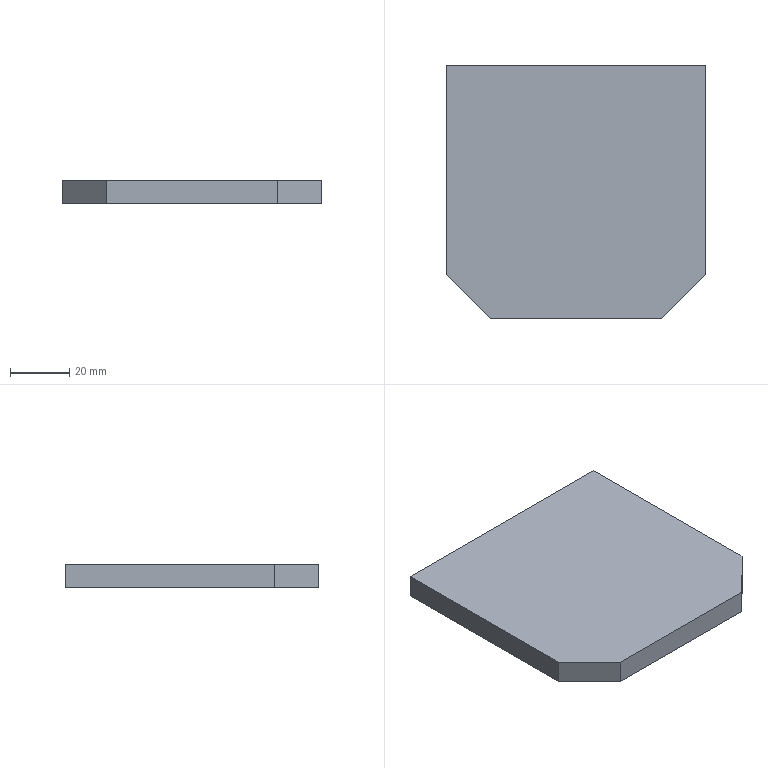Part | STEP file | 400 | 1 solid | 8 faces | box 88 x 86 x 8 mm | volume 58744 mm3 | plane 8
STEP:
#1=CARTESIAN_POINT('',(-29.,-94.,725.));
#2=VERTEX_POINT('',#1);
#3=CARTESIAN_POINT('',(-29.,-94.,717.));
#4=VERTEX_POINT('',#3);
#5=CARTESIAN_POINT('',(-29.,-94.,725.));
#6=DIRECTION('',(0.,0.,-1.));
#7=VECTOR('',#6,1000.);
#8=LINE('',#5,#7);
#9=EDGE_CURVE('',#2,#4,#8,.T.);
#10=ORIENTED_EDGE('',*,*,#9,.T.);
#11=CARTESIAN_POINT('',(29.,-94.,717.));
#12=VERTEX_POINT('',#11);
#13=CARTESIAN_POINT('',(-29.,-94.,717.));
#14=DIRECTION('',(1.,0.,0.));
#15=VECTOR('',#14,1000.);
#16=LINE('',#13,#15);
#17=EDGE_CURVE('',#4,#12,#16,.T.);
#18=ORIENTED_EDGE('',*,*,#17,.T.);
#19=CARTESIAN_POINT('',(29.,-94.,725.));
#20=VERTEX_POINT('',#19);
#21=CARTESIAN_POINT('',(29.,-94.,725.));
#22=DIRECTION('',(0.,0.,-1.));
#23=VECTOR('',#22,1000.);
#24=LINE('',#21,#23);
#25=EDGE_CURVE('',#20,#12,#24,.T.);
#26=ORIENTED_EDGE('',*,*,#25,.F.);
#27=CARTESIAN_POINT('',(-29.,-94.,725.));
#28=DIRECTION('',(1.,0.,0.));
#29=VECTOR('',#28,1000.);
#30=LINE('',#27,#29);
#31=EDGE_CURVE('',#2,#20,#30,.T.);
#32=ORIENTED_EDGE('',*,*,#31,.F.);
#33=EDGE_LOOP('',(#10,#18,#26,#32));
#34=FACE_OUTER_BOUND('',#33,.T.);
#35=CARTESIAN_POINT('',(-29.,-94.,717.));
#36=DIRECTION('',(0.,-1.,0.));
#37=DIRECTION('',(0.,0.,-1.));
#38=AXIS2_PLACEMENT_3D('',#35,#36,#37);
#39=PLANE('',#38);
#40=ADVANCED_FACE('',(#34),#39,.T.);
#41=CARTESIAN_POINT('',(-44.,-79.,725.));
#42=VERTEX_POINT('',#41);
#43=CARTESIAN_POINT('',(-44.,-79.,717.));
#44=VERTEX_POINT('',#43);
#45=CARTESIAN_POINT('',(-44.,-79.,725.));
#46=DIRECTION('',(0.,0.,-1.));
#47=VECTOR('',#46,1000.);
#48=LINE('',#45,#47);
#49=EDGE_CURVE('',#42,#44,#48,.T.);
#50=ORIENTED_EDGE('',*,*,#49,.T.);
#51=CARTESIAN_POINT('',(-29.,-94.,717.));
#52=DIRECTION('',(-0.7071,0.7071,0.));
#53=VECTOR('',#52,1000.);
#54=LINE('',#51,#53);
#55=EDGE_CURVE('',#4,#44,#54,.T.);
#56=ORIENTED_EDGE('',*,*,#55,.F.);
#57=ORIENTED_EDGE('',*,*,#9,.F.);
#58=CARTESIAN_POINT('',(-44.,-79.,725.));
#59=DIRECTION('',(0.7071,-0.7071,0.));
#60=VECTOR('',#59,1000.);
#61=LINE('',#58,#60);
#62=EDGE_CURVE('',#42,#2,#61,.T.);
#63=ORIENTED_EDGE('',*,*,#62,.F.);
#64=EDGE_LOOP('',(#50,#56,#57,#63));
#65=FACE_OUTER_BOUND('',#64,.T.);
#66=CARTESIAN_POINT('',(-44.,-79.,717.));
#67=DIRECTION('',(-0.7071,-0.7071,0.));
#68=DIRECTION('',(-0.7071,0.7071,0.));
#69=AXIS2_PLACEMENT_3D('',#66,#67,#68);
#70=PLANE('',#69);
#71=ADVANCED_FACE('',(#65),#70,.T.);
#72=CARTESIAN_POINT('',(44.,-79.,725.));
#73=VERTEX_POINT('',#72);
#74=CARTESIAN_POINT('',(44.,-79.,717.));
#75=VERTEX_POINT('',#74);
#76=CARTESIAN_POINT('',(44.,-79.,725.));
#77=DIRECTION('',(0.,0.,-1.));
#78=VECTOR('',#77,1000.);
#79=LINE('',#76,#78);
#80=EDGE_CURVE('',#73,#75,#79,.T.);
#81=ORIENTED_EDGE('',*,*,#80,.T.);
#82=CARTESIAN_POINT('',(44.,-8.,717.));
#83=VERTEX_POINT('',#82);
#84=CARTESIAN_POINT('',(44.,-8.,717.));
#85=DIRECTION('',(0.,-1.,0.));
#86=VECTOR('',#85,1000.);
#87=LINE('',#84,#86);
#88=EDGE_CURVE('',#83,#75,#87,.T.);
#89=ORIENTED_EDGE('',*,*,#88,.F.);
#90=CARTESIAN_POINT('',(44.,-8.,725.));
#91=VERTEX_POINT('',#90);
#92=CARTESIAN_POINT('',(44.,-8.,725.));
#93=DIRECTION('',(0.,0.,-1.));
#94=VECTOR('',#93,1000.);
#95=LINE('',#92,#94);
#96=EDGE_CURVE('',#91,#83,#95,.T.);
#97=ORIENTED_EDGE('',*,*,#96,.F.);
#98=CARTESIAN_POINT('',(44.,-79.,725.));
#99=DIRECTION('',(0.,1.,0.));
#100=VECTOR('',#99,1000.);
#101=LINE('',#98,#100);
#102=EDGE_CURVE('',#73,#91,#101,.T.);
#103=ORIENTED_EDGE('',*,*,#102,.F.);
#104=EDGE_LOOP('',(#81,#89,#97,#103));
#105=FACE_OUTER_BOUND('',#104,.T.);
#106=CARTESIAN_POINT('',(44.,-79.,717.));
#107=DIRECTION('',(1.,0.,0.));
#108=DIRECTION('',(0.,1.,0.));
#109=AXIS2_PLACEMENT_3D('',#106,#107,#108);
#110=PLANE('',#109);
#111=ADVANCED_FACE('',(#105),#110,.T.);
#112=ORIENTED_EDGE('',*,*,#96,.T.);
#113=CARTESIAN_POINT('',(-44.,-8.,717.));
#114=VERTEX_POINT('',#113);
#115=CARTESIAN_POINT('',(-44.,-8.,717.));
#116=DIRECTION('',(1.,0.,0.));
#117=VECTOR('',#116,1000.);
#118=LINE('',#115,#117);
#119=EDGE_CURVE('',#114,#83,#118,.T.);
#120=ORIENTED_EDGE('',*,*,#119,.F.);
#121=CARTESIAN_POINT('',(-44.,-8.,725.));
#122=VERTEX_POINT('',#121);
#123=CARTESIAN_POINT('',(-44.,-8.,725.));
#124=DIRECTION('',(0.,0.,-1.));
#125=VECTOR('',#124,1000.);
#126=LINE('',#123,#125);
#127=EDGE_CURVE('',#122,#114,#126,.T.);
#128=ORIENTED_EDGE('',*,*,#127,.F.);
#129=CARTESIAN_POINT('',(44.,-8.,725.));
#130=DIRECTION('',(-1.,0.,0.));
#131=VECTOR('',#130,1000.);
#132=LINE('',#129,#131);
#133=EDGE_CURVE('',#91,#122,#132,.T.);
#134=ORIENTED_EDGE('',*,*,#133,.F.);
#135=EDGE_LOOP('',(#112,#120,#128,#134));
#136=FACE_OUTER_BOUND('',#135,.T.);
#137=CARTESIAN_POINT('',(29.,-8.,717.));
#138=DIRECTION('',(0.,1.,0.));
#139=DIRECTION('',(1.,0.,0.));
#140=AXIS2_PLACEMENT_3D('',#137,#138,#139);
#141=PLANE('',#140);
#142=ADVANCED_FACE('',(#136),#141,.T.);
#143=ORIENTED_EDGE('',*,*,#88,.T.);
#144=CARTESIAN_POINT('',(44.,-79.,717.));
#145=DIRECTION('',(-0.7071,-0.7071,0.));
#146=VECTOR('',#145,1000.);
#147=LINE('',#144,#146);
#148=EDGE_CURVE('',#75,#12,#147,.T.);
#149=ORIENTED_EDGE('',*,*,#148,.T.);
#150=ORIENTED_EDGE('',*,*,#17,.F.);
#151=ORIENTED_EDGE('',*,*,#55,.T.);
#152=CARTESIAN_POINT('',(-44.,-8.,717.));
#153=DIRECTION('',(0.,-1.,0.));
#154=VECTOR('',#153,1000.);
#155=LINE('',#152,#154);
#156=EDGE_CURVE('',#114,#44,#155,.T.);
#157=ORIENTED_EDGE('',*,*,#156,.F.);
#158=ORIENTED_EDGE('',*,*,#119,.T.);
#159=EDGE_LOOP('',(#143,#149,#150,#151,#157,#158));
#160=FACE_OUTER_BOUND('',#159,.T.);
#161=CARTESIAN_POINT('',(0.,0.,717.));
#162=DIRECTION('',(0.,0.,-1.));
#163=DIRECTION('',(0.,-1.,0.));
#164=AXIS2_PLACEMENT_3D('',#161,#162,#163);
#165=PLANE('',#164);
#166=ADVANCED_FACE('',(#160),#165,.T.);
#167=ORIENTED_EDGE('',*,*,#49,.F.);
#168=CARTESIAN_POINT('',(-44.,-8.,725.));
#169=DIRECTION('',(0.,-1.,0.));
#170=VECTOR('',#169,1000.);
#171=LINE('',#168,#170);
#172=EDGE_CURVE('',#122,#42,#171,.T.);
#173=ORIENTED_EDGE('',*,*,#172,.F.);
#174=ORIENTED_EDGE('',*,*,#127,.T.);
#175=ORIENTED_EDGE('',*,*,#156,.T.);
#176=EDGE_LOOP('',(#167,#173,#174,#175));
#177=FACE_OUTER_BOUND('',#176,.T.);
#178=CARTESIAN_POINT('',(-44.,-23.,717.));
#179=DIRECTION('',(-1.,0.,0.));
#180=DIRECTION('',(0.,0.,1.));
#181=AXIS2_PLACEMENT_3D('',#178,#179,#180);
#182=PLANE('',#181);
#183=ADVANCED_FACE('',(#177),#182,.T.);
#184=ORIENTED_EDGE('',*,*,#62,.T.);
#185=ORIENTED_EDGE('',*,*,#31,.T.);
#186=CARTESIAN_POINT('',(29.,-94.,725.));
#187=DIRECTION('',(0.7071,0.7071,0.));
#188=VECTOR('',#187,1000.);
#189=LINE('',#186,#188);
#190=EDGE_CURVE('',#20,#73,#189,.T.);
#191=ORIENTED_EDGE('',*,*,#190,.T.);
#192=ORIENTED_EDGE('',*,*,#102,.T.);
#193=ORIENTED_EDGE('',*,*,#133,.T.);
#194=ORIENTED_EDGE('',*,*,#172,.T.);
#195=EDGE_LOOP('',(#184,#185,#191,#192,#193,#194));
#196=FACE_OUTER_BOUND('',#195,.T.);
#197=CARTESIAN_POINT('',(0.,0.,725.));
#198=DIRECTION('',(0.,0.,-1.));
#199=DIRECTION('',(0.,-1.,0.));
#200=AXIS2_PLACEMENT_3D('',#197,#198,#199);
#201=PLANE('',#200);
#202=ADVANCED_FACE('',(#196),#201,.F.);
#203=ORIENTED_EDGE('',*,*,#25,.T.);
#204=ORIENTED_EDGE('',*,*,#148,.F.);
#205=ORIENTED_EDGE('',*,*,#80,.F.);
#206=ORIENTED_EDGE('',*,*,#190,.F.);
#207=EDGE_LOOP('',(#203,#204,#205,#206));
#208=FACE_OUTER_BOUND('',#207,.T.);
#209=CARTESIAN_POINT('',(29.,-94.,717.));
#210=DIRECTION('',(0.7071,-0.7071,0.));
#211=DIRECTION('',(0.,0.,-1.));
#212=AXIS2_PLACEMENT_3D('',#209,#210,#211);
#213=PLANE('',#212);
#214=ADVANCED_FACE('',(#208),#213,.T.);
#215=CLOSED_SHELL('',(#40,#71,#111,#142,#166,#183,#202,#214));
#216=MANIFOLD_SOLID_BREP('',#215);
#217=CARTESIAN_POINT('',(0.,0.,0.));
#218=DIRECTION('',(0.,0.,1.));
#219=DIRECTION('',(1.,0.,0.));
#220=AXIS2_PLACEMENT_3D('',#217,#218,#219);
#221=(LENGTH_UNIT()NAMED_UNIT(*)SI_UNIT(.MILLI.,.METRE.));
#222=UNCERTAINTY_MEASURE_WITH_UNIT(LENGTH_MEASURE(0.00001),#221,'','');
#223=(NAMED_UNIT(*)PLANE_ANGLE_UNIT()SI_UNIT($,.RADIAN.));
#224=(NAMED_UNIT(*)SI_UNIT($,.STERADIAN.)SOLID_ANGLE_UNIT());
#225=(GEOMETRIC_REPRESENTATION_CONTEXT(3)GLOBAL_UNCERTAINTY_ASSIGNED_CONTEXT((#222))GLOBAL_UNIT_ASSIGNED_CONTEXT((#221,#223,#224))REPRESENTATION_CONTEXT('',''));
#226=ADVANCED_BREP_SHAPE_REPRESENTATION('',(#216,#220),#225);